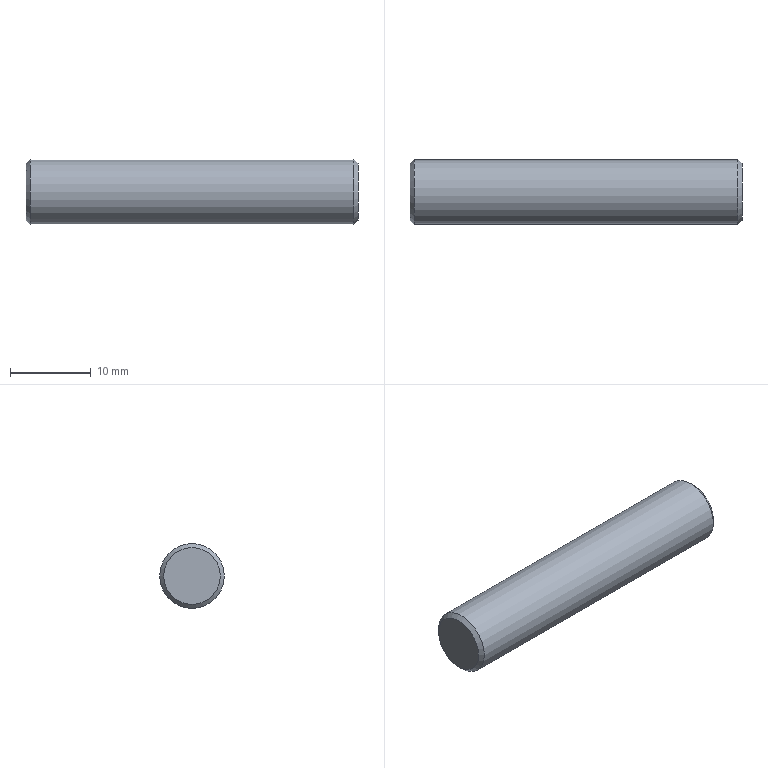Part | NX | features solid 2 | 1 solid | 5 faces | box 41 x 8 x 8 mm | volume 2055 mm3 | plane 2 | cone 2 | cylinder 1 | commonest cylinder face diameters 8 x1
STEP:
#1=CARTESIAN_POINT('',(255.5,-222.,31.5));
#2=VERTEX_POINT('',#1);
#3=CARTESIAN_POINT('',(255.5,-218.,31.5));
#4=DIRECTION('',(-1.,0.,0.));
#5=DIRECTION('',(0.,-1.,0.));
#6=AXIS2_PLACEMENT_3D('',#3,#4,#5);
#7=CIRCLE('',#6,4.);
#8=EDGE_CURVE('',#2,#2,#7,.T.);
#9=ORIENTED_EDGE('',*,*,#8,.T.);
#10=EDGE_LOOP('',(#9));
#11=FACE_BOUND('',#10,.T.);
#12=CARTESIAN_POINT('',(215.5,-214.,31.5));
#13=VERTEX_POINT('',#12);
#14=CARTESIAN_POINT('',(215.5,-218.,31.5));
#15=DIRECTION('',(1.,0.,0.));
#16=DIRECTION('',(0.,1.,0.));
#17=AXIS2_PLACEMENT_3D('',#14,#15,#16);
#18=CIRCLE('',#17,4.);
#19=EDGE_CURVE('',#13,#13,#18,.T.);
#20=ORIENTED_EDGE('',*,*,#19,.T.);
#21=EDGE_LOOP('',(#20));
#22=FACE_BOUND('',#21,.T.);
#23=CARTESIAN_POINT('',(256.,-218.,31.5));
#24=DIRECTION('',(-1.,0.,0.));
#25=DIRECTION('',(0.,1.,0.));
#26=AXIS2_PLACEMENT_3D('',#23,#24,#25);
#27=CYLINDRICAL_SURFACE('',#26,4.);
#28=ADVANCED_FACE('',(#11,#22),#27,.T.);
#29=CARTESIAN_POINT('',(256.,-221.5,31.5));
#30=VERTEX_POINT('',#29);
#31=CARTESIAN_POINT('',(256.,-218.,31.5));
#32=DIRECTION('',(1.,0.,0.));
#33=DIRECTION('',(0.,-1.,0.));
#34=AXIS2_PLACEMENT_3D('',#31,#32,#33);
#35=CIRCLE('',#34,3.5);
#36=EDGE_CURVE('',#30,#30,#35,.T.);
#37=ORIENTED_EDGE('',*,*,#36,.T.);
#38=EDGE_LOOP('',(#37));
#39=FACE_BOUND('',#38,.T.);
#40=CARTESIAN_POINT('',(256.,-218.,31.5));
#41=DIRECTION('',(-1.,0.,0.));
#42=DIRECTION('',(0.,1.,0.));
#43=AXIS2_PLACEMENT_3D('',#40,#41,#42);
#44=PLANE('',#43);
#45=ADVANCED_FACE('',(#39),#44,.F.);
#46=CARTESIAN_POINT('',(215.,-221.5,31.5));
#47=VERTEX_POINT('',#46);
#48=CARTESIAN_POINT('',(215.,-218.,31.5));
#49=DIRECTION('',(-1.,0.,0.));
#50=DIRECTION('',(0.,-1.,0.));
#51=AXIS2_PLACEMENT_3D('',#48,#49,#50);
#52=CIRCLE('',#51,3.5);
#53=EDGE_CURVE('',#47,#47,#52,.T.);
#54=ORIENTED_EDGE('',*,*,#53,.T.);
#55=EDGE_LOOP('',(#54));
#56=FACE_BOUND('',#55,.T.);
#57=CARTESIAN_POINT('',(215.,-218.,31.5));
#58=DIRECTION('',(-1.,0.,0.));
#59=DIRECTION('',(0.,1.,0.));
#60=AXIS2_PLACEMENT_3D('',#57,#58,#59);
#61=PLANE('',#60);
#62=ADVANCED_FACE('',(#56),#61,.T.);
#63=ORIENTED_EDGE('',*,*,#36,.F.);
#64=EDGE_LOOP('',(#63));
#65=FACE_BOUND('',#64,.T.);
#66=ORIENTED_EDGE('',*,*,#8,.F.);
#67=EDGE_LOOP('',(#66));
#68=FACE_BOUND('',#67,.T.);
#69=CARTESIAN_POINT('',(255.5,-218.,31.5));
#70=DIRECTION('',(-1.,0.,0.));
#71=DIRECTION('',(0.,1.,0.));
#72=AXIS2_PLACEMENT_3D('',#69,#70,#71);
#73=CONICAL_SURFACE('',#72,4.,0.7854);
#74=ADVANCED_FACE('',(#65,#68),#73,.T.);
#75=ORIENTED_EDGE('',*,*,#19,.F.);
#76=EDGE_LOOP('',(#75));
#77=FACE_BOUND('',#76,.T.);
#78=ORIENTED_EDGE('',*,*,#53,.F.);
#79=EDGE_LOOP('',(#78));
#80=FACE_BOUND('',#79,.T.);
#81=CARTESIAN_POINT('',(215.,-218.,31.5));
#82=DIRECTION('',(1.,0.,0.));
#83=DIRECTION('',(0.,-1.,0.));
#84=AXIS2_PLACEMENT_3D('',#81,#82,#83);
#85=CONICAL_SURFACE('',#84,3.5,0.7854);
#86=ADVANCED_FACE('',(#77,#80),#85,.T.);
#87=CLOSED_SHELL('',(#28,#45,#62,#74,#86));
#88=MANIFOLD_SOLID_BREP('',#87);
#89=(LENGTH_UNIT()NAMED_UNIT(*)SI_UNIT(.MILLI.,.METRE.));
#90=UNCERTAINTY_MEASURE_WITH_UNIT(LENGTH_MEASURE(0.00001),#89,'','');
#91=(NAMED_UNIT(*)PLANE_ANGLE_UNIT()SI_UNIT($,.RADIAN.));
#92=(NAMED_UNIT(*)SI_UNIT($,.STERADIAN.)SOLID_ANGLE_UNIT());
#93=(GEOMETRIC_REPRESENTATION_CONTEXT(3)GLOBAL_UNCERTAINTY_ASSIGNED_CONTEXT((#90))GLOBAL_UNIT_ASSIGNED_CONTEXT((#89,#91,#92))REPRESENTATION_CONTEXT('',''));
#94=ADVANCED_BREP_SHAPE_REPRESENTATION('',(#88),#93);